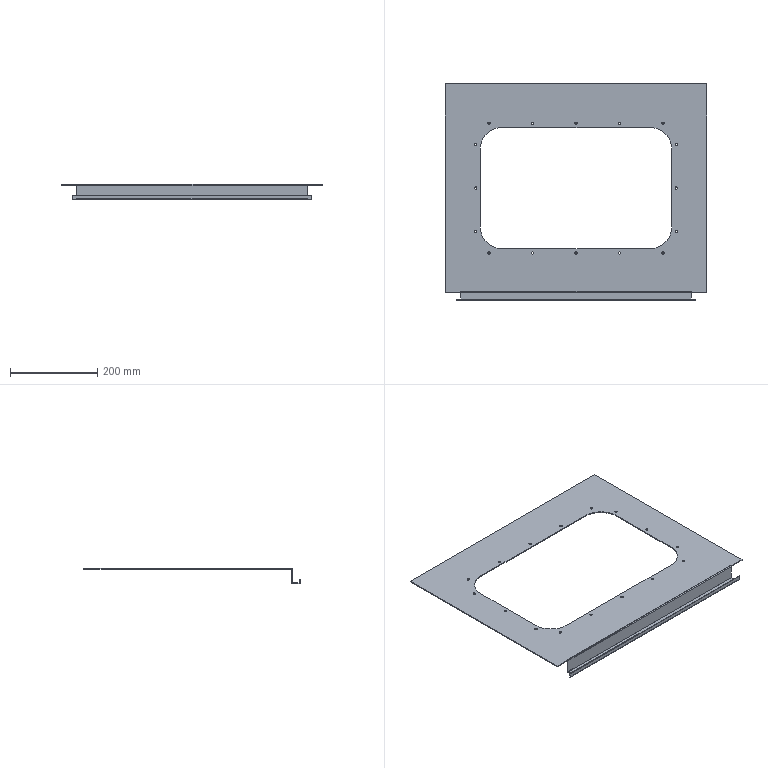Part | SolidWorks | features MoveFace 2, BaseBody 1 | 1 solid | 74 faces | box 600 x 496 x 35 mm | volume 393982 mm3 | cylinder 42 | plane 32 | commonest cylinder face diameters 5.3 x32 100 x4 0.2 x3 4.2 x3